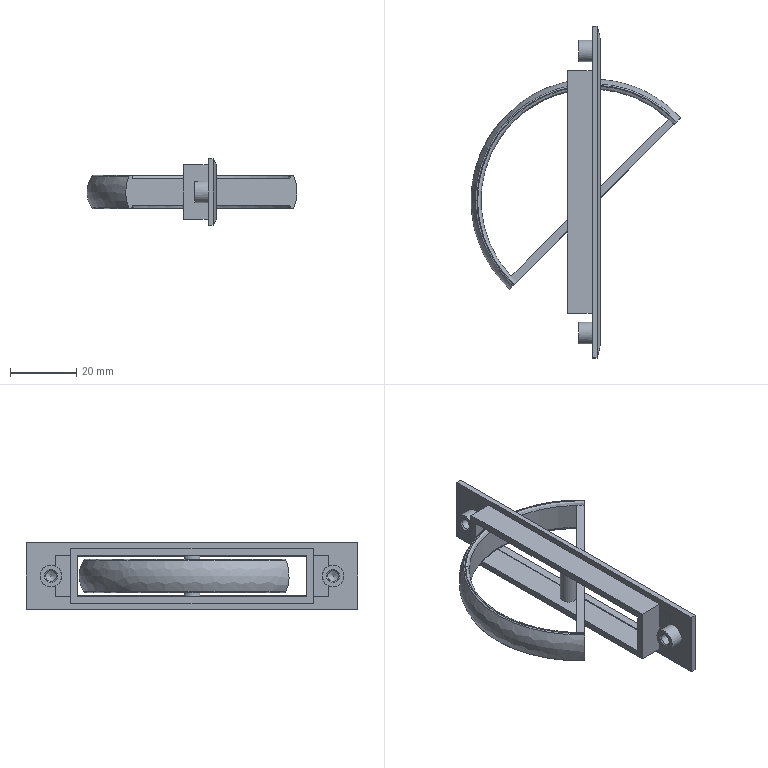Part | STEP file | LS707 rotary concealed handle | 1 solid | 56 faces | box 63.292 x 100 x 20 mm | volume 9779 mm3 | plane 41 | cylinder 6 | spline 5 | cone 4 | commonest cylinder face diameters 3.242 x2 6.5 x2 5 x1 67 x1